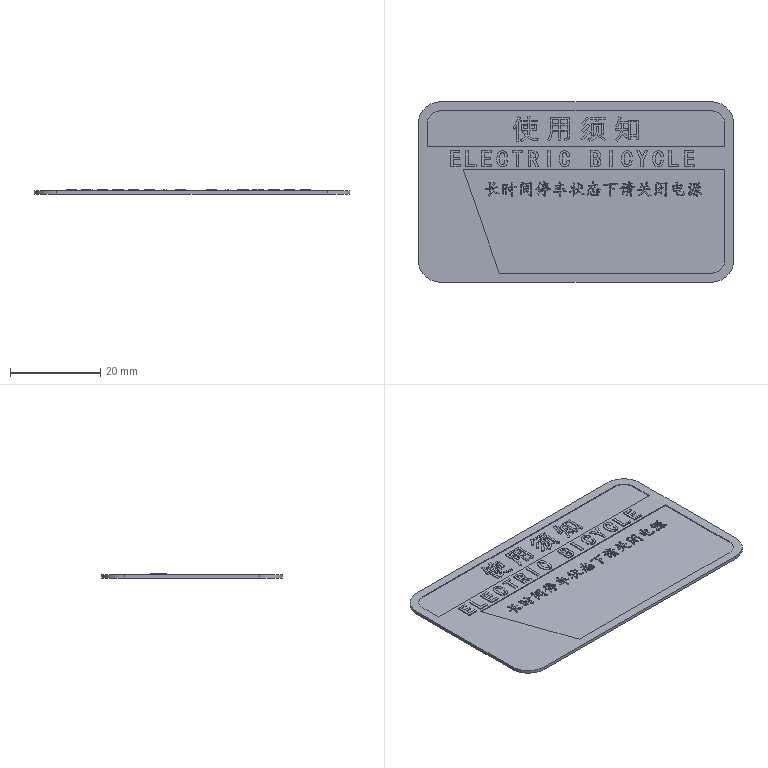Part | SolidWorks | features BaseBody 16 | 16 solids | 638 faces | box 70 x 40 x 0.9 mm | volume 1612 mm3 | spline 318 | plane 313 | cylinder 7 | commonest cylinder face diameters 10 x4 6 x3